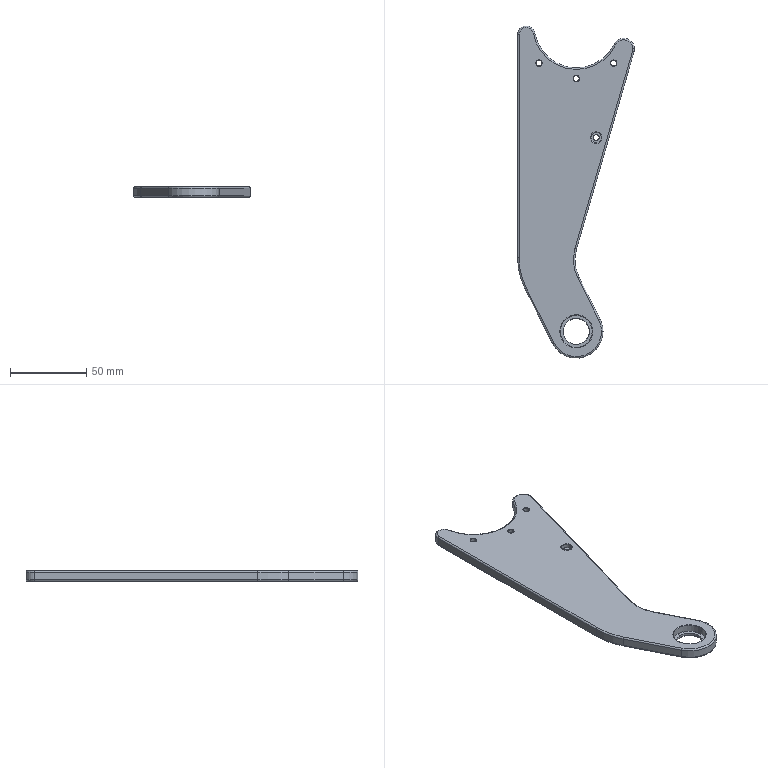Part | SolidWorks | features Fillet 5, ICE 4, Extrusion 1 | 1 solid | 101 faces | box 76.423 x 217.462 x 7 mm | volume 66603 mm3 | torus 56 | cylinder 34 | plane 11 | commonest cylinder face diameters 2 x8 3.7 x8 7 x8 17 x2 21.15 x2 11.404 x1